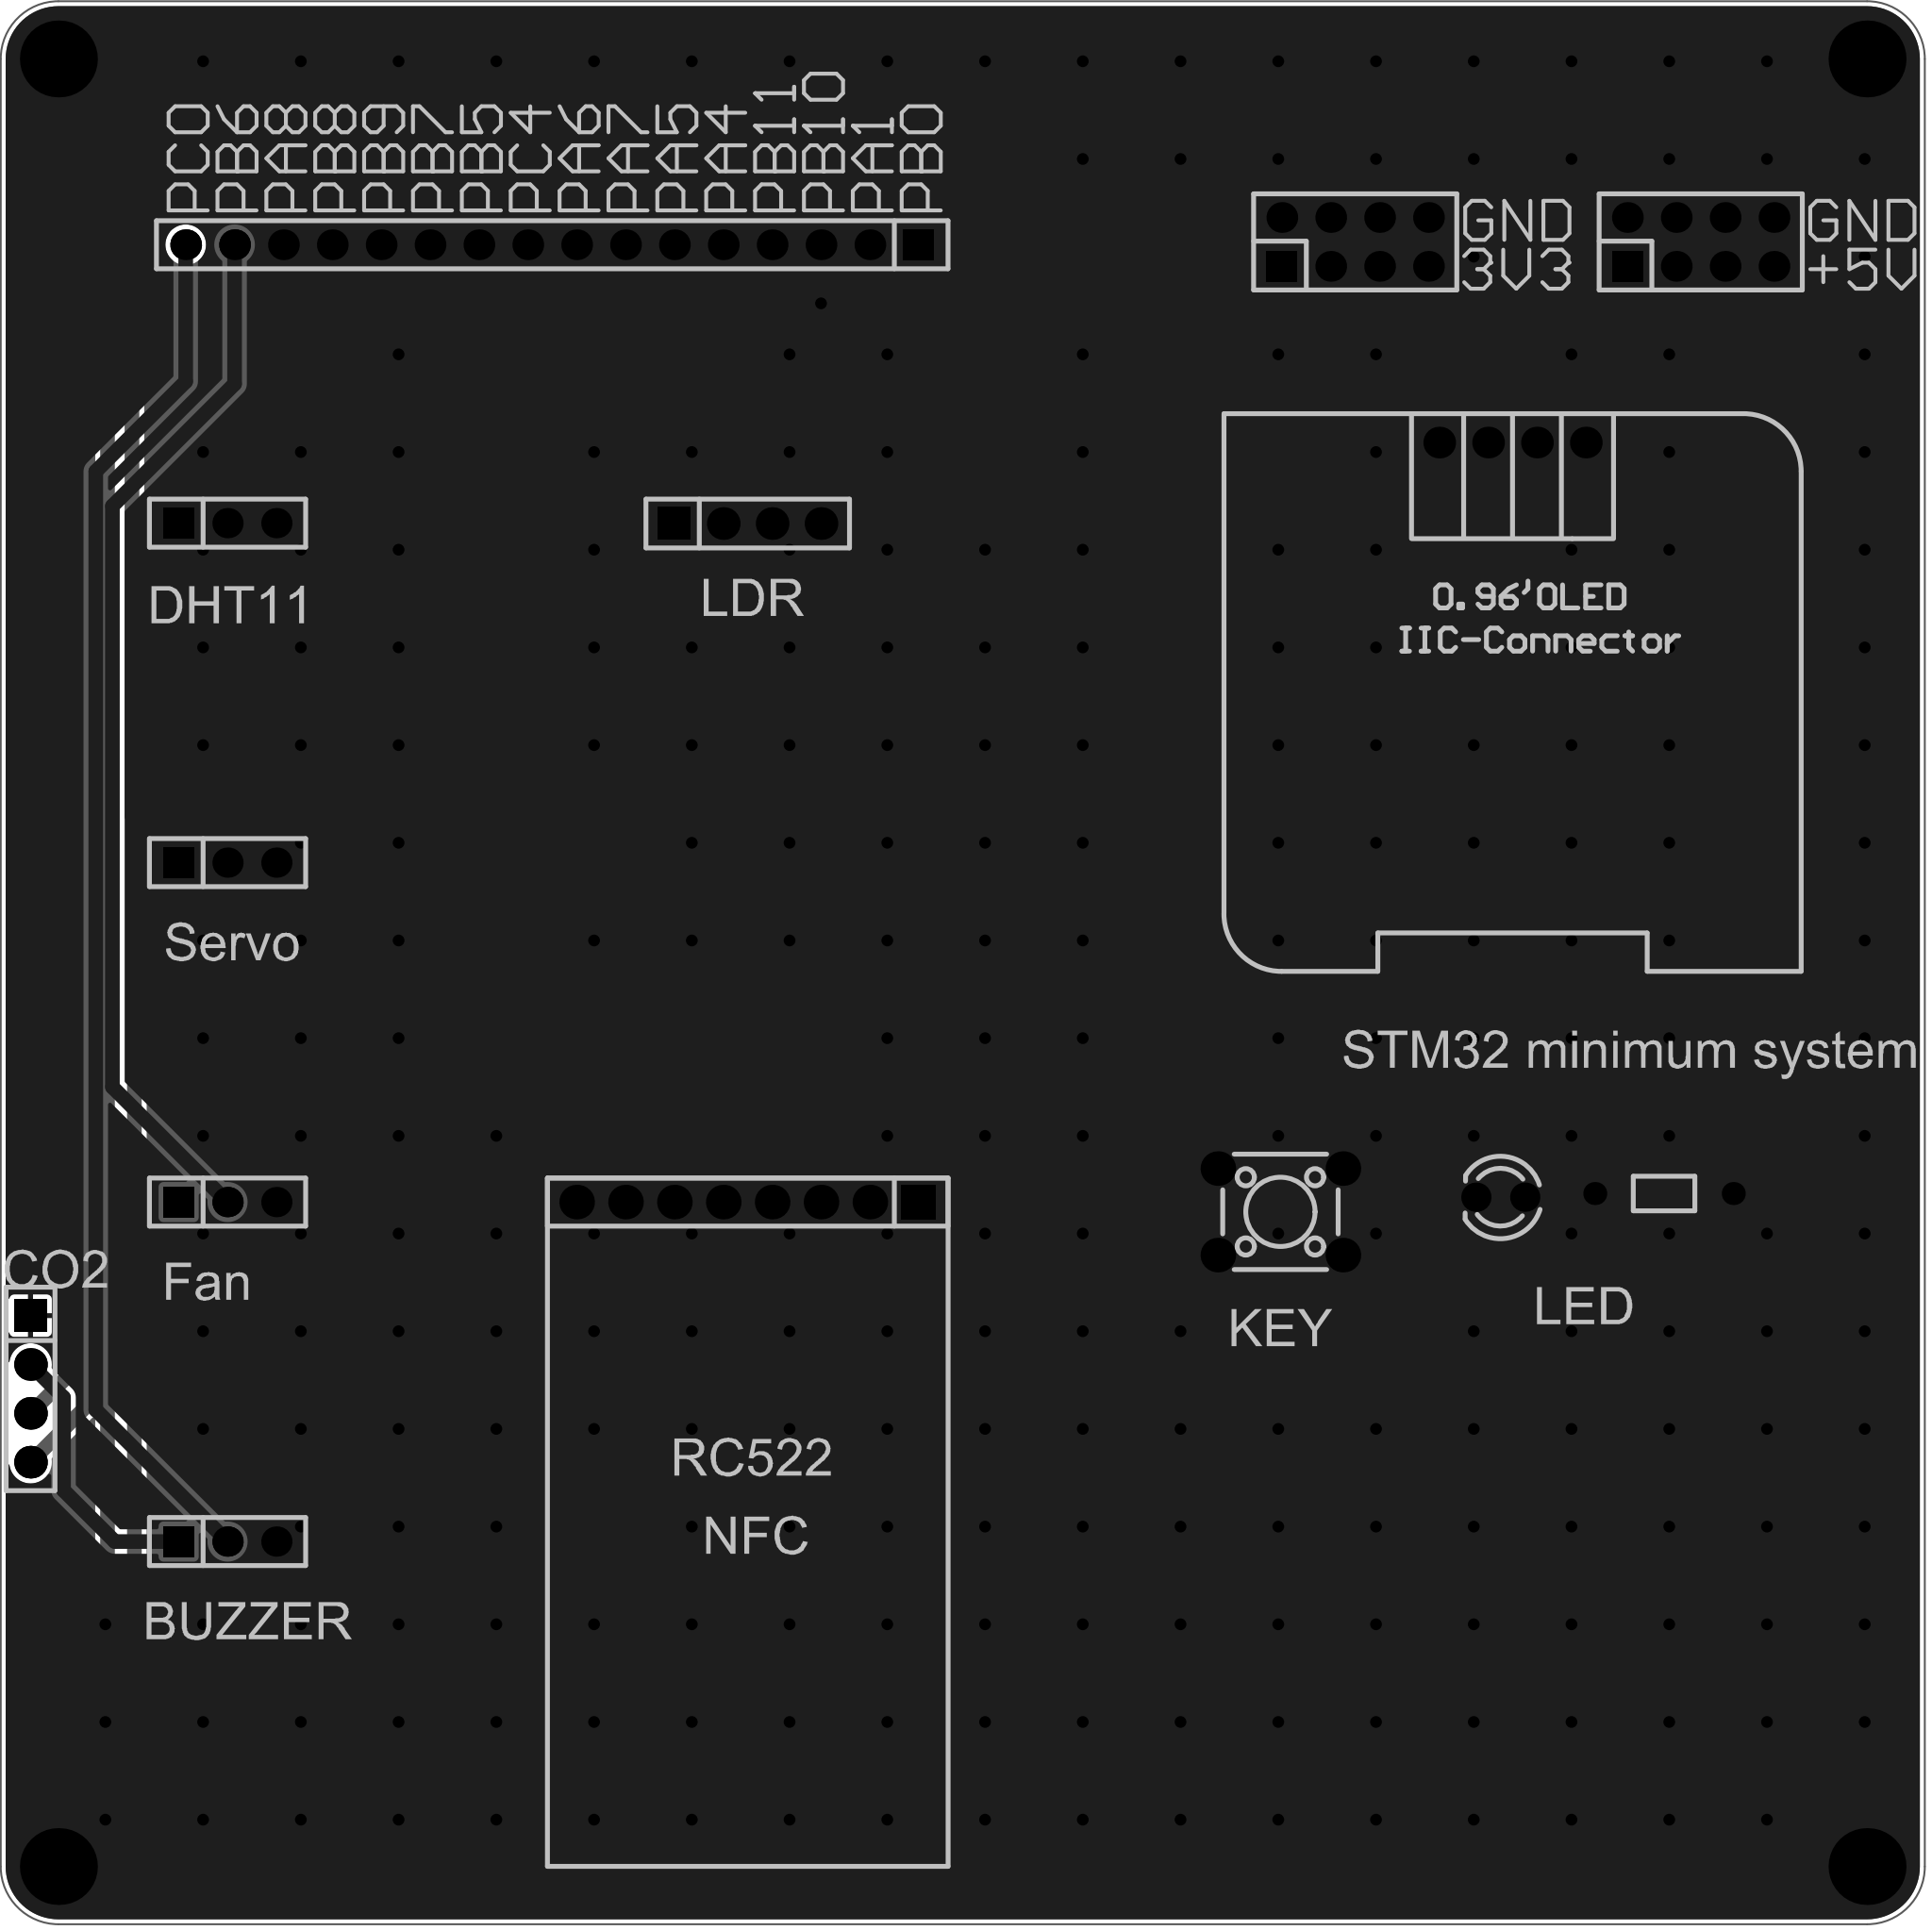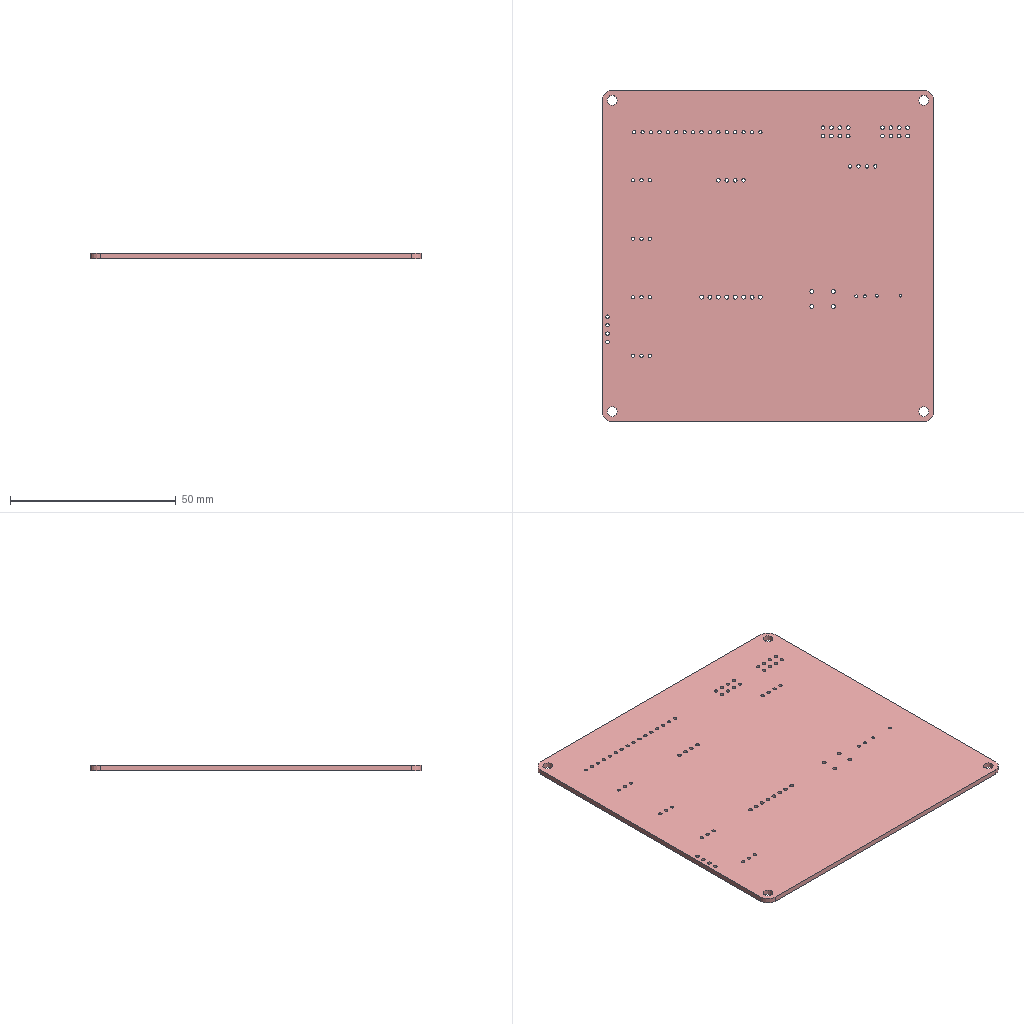Circuit board layout | Altium Designer | box 100 x 100 x 1.6 mm
Layer stack:
# Altium Designer layer stack of  (unit mm; dielectric type: 0 none, 1 core, 2 prepreg, 3 surface material)
index,name,kind,layer,copper_thickness_mm,dielectric_type,dielectric_thickness_mm,dielectric_material,dielectric_constant
0,Top Paste Mask Layer,other,,,,,,
1,Top Silkscreen Layer,other,,,,,,
2,Top Solder Mask Layer,dielectric,,,3,0.01,,3.3
3,Top Layer,copper,Top Layer,0.035,,,,
4,Dielectric1,dielectric,,,3,1.51,FR4,4.5
5,Bottom Layer,copper,Bottom Layer,0.035,,,,
6,Bottom Solder Mask Layer,dielectric,,,3,0.01,,3.3
7,Bottom Silkscreen Layer,other,,,,,,
8,Bottom Paste Mask Layer,other,,,,,,
# drill layer pairs: low layer,high layer
drill_pair,Top Layer,Bottom Layer
Part placement:
Designator,Comment,Layer,Footprint,Center-X(mm),Center-Y(mm),Rotation
H6,,TopLayer,HDR-TH_4P-P2.54-V-F,118.491,151.745,0
H1,,TopLayer,HDR-TH_8P-P2.54-V-F-1,118.491,116.459,180
H2,,TopLayer,HDR-TH_3P-P2.54-V-F,91.455,134.112,0
H3,,TopLayer,HDR-TH_3P-P2.54-V-F,91.455,151.765,0
H4,,TopLayer,HDR-TH_3P-P2.54-V-F,91.455,116.459,0
H5,,TopLayer,HDR-TH_4P-P2.54-V-F,81.216,106.743,270
H8,,TopLayer,HDR-TH_8P-P2.54-V-F-R2-C4-S2.54-1,150.063,166.39,0
H9,,TopLayer,HDR-TH_8P-P2.54-V-F-R2-C4-S2.54-1,168.021,166.39,0
H18,,TopLayer,HDR-TH_3P-P2.54-V-F,91.455,98.806,0
LED1,,TopLayer,LED_TH-3mm,157.607,116.713,180
OLED1,,TopLayer,0.96OLED_4P,158.242,155.956,0
SW1,,TopLayer,SW-TH_4P-L6.0-W6.0-P4.50-LS6.5,146.177,115.951,0
R1,300,TopLayer,Res_1/8W,166.116,116.903,0
H7,,TopLayer,HDR-TH_16P-P2.54-V-F,108.331,166.243,180
Pad and via stacks:
# Altium Designer via and pad stacks of  (unit mm). Each distinct definition once, with the count of objects using it.
# via: kind,start_layer,end_layer,hole_mm,diameter_mm,mode(0 simple;1 top-mid-bottom;2 full stack),diameter_per_layer,count,example_net
# pad: kind,layer,hole_mm,hole_type(0 round;1 square;2 slot),plating,top_size,top_shape(1 round;2 rect;3 octagon;9 rounded rect),mid_size,bottom_size,mode,footprint,size_per_layer,count,example
pad,Multi-Layer,3,0,plated,4x4,1,4x4,4x4,0,,,4,1
pad,Multi-Layer,1.1,0,plated,1.7x1.7,2,1.7x1.7,1.7x1.7,0,HDR-TH_4P-P2.54-V-F,,2,H6.1
pad,Multi-Layer,1.1,0,plated,1.7x1.7,1,1.7x1.7,1.7x1.7,0,HDR-TH_4P-P2.54-V-F,,6,H6.2
pad,Multi-Layer,1.2,0,plated,1.8x1.8,2,1.8x1.8,1.8x1.8,0,HDR-TH_8P-P2.54-V-F-1,,1,H1.1
pad,Multi-Layer,1.2,0,plated,1.8x1.8,1,1.8x1.8,1.8x1.8,0,HDR-TH_8P-P2.54-V-F-1,,7,H1.2
pad,Multi-Layer,1.02,0,plated,1.575x1.575,1,1.575x1.575,1.575x1.575,0,HDR-TH_3P-P2.54-V-F,,8,H2.3
pad,Multi-Layer,1.02,0,plated,1.575x1.575,2,1.575x1.575,1.575x1.575,0,HDR-TH_3P-P2.54-V-F,,4,H2.1
pad,Multi-Layer,1.1,0,plated,1.6x1.6,2,1.6x1.6,1.6x1.6,0,HDR-TH_8P-P2.54-V-F-R2-C4-S2.54-1,,2,H8.1
pad,Multi-Layer,1.1,0,plated,1.6x1.6,1,1.6x1.6,1.6x1.6,0,HDR-TH_8P-P2.54-V-F-R2-C4-S2.54-1,,14,H8.2
pad,Multi-Layer,0.9144,0,plated,1.524x1.524,1,1.524x1.524,1.524x1.524,0,LED_TH-3mm,,2,LED1.1
pad,Multi-Layer,1,0,plated,1.65x1.65,1,1.65x1.65,1.65x1.65,0,0.96OLED_4P,,4,OLED1.4
pad,Multi-Layer,1.2,0,plated,1.8x1.8,1,1.8x1.8,1.8x1.8,0,SW-TH_4P-L6.0-W6.0-P4.50-LS6.5,,4,SW1.1
pad,Multi-Layer,0.8001,0,plated,1.199x1.199,1,1.199x1.199,1.199x1.199,0,Res_1/8W,,2,R1.1
pad,Multi-Layer,1,0,plated,1.6x1.6,2,1.6x1.6,1.6x1.6,0,HDR-TH_16P-P2.54-V-F,,1,H7.1
pad,Multi-Layer,1,0,plated,1.6x1.6,1,1.6x1.6,1.6x1.6,0,HDR-TH_16P-P2.54-V-F,,15,H7.2
via,Top Layer,Bottom Layer,0.3048,0.61,0,,266,GND
Copper pours:
name,layer,net,type(0 solid;1 hatched;2 none)
Bottom Layer-GND,Bottom Layer,GND,0
Top Layer-GND,Top Layer,GND,0